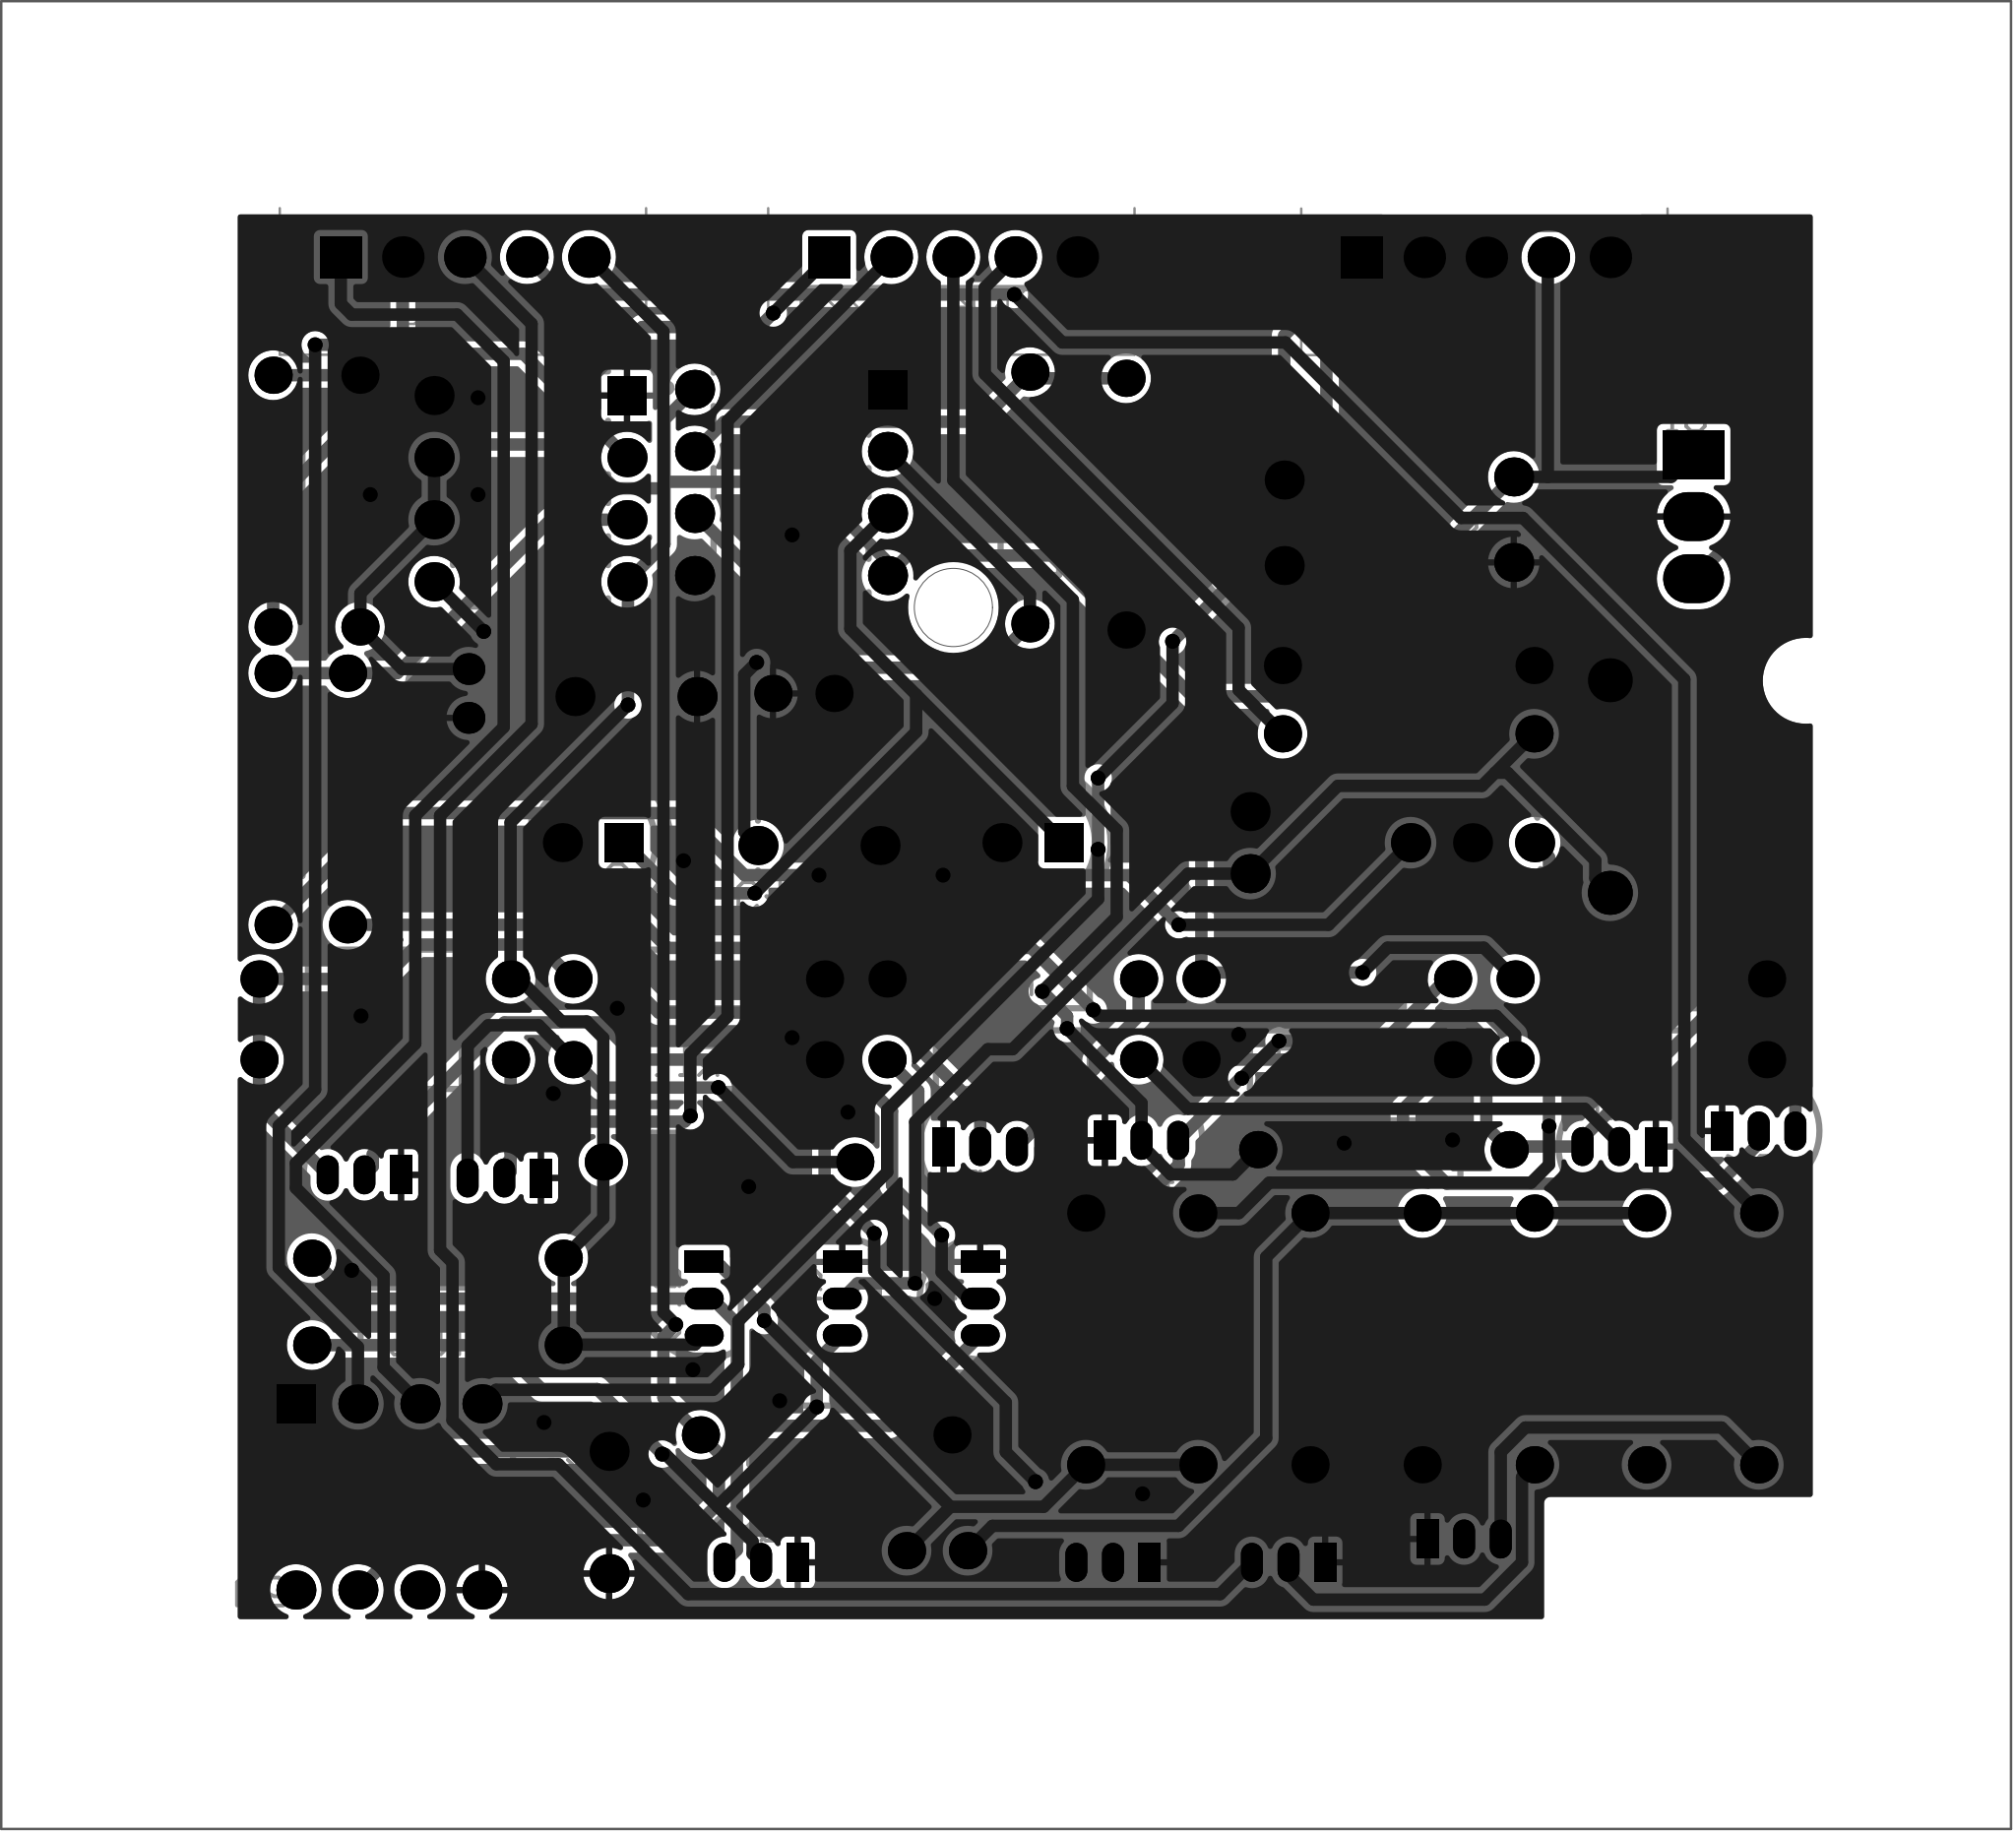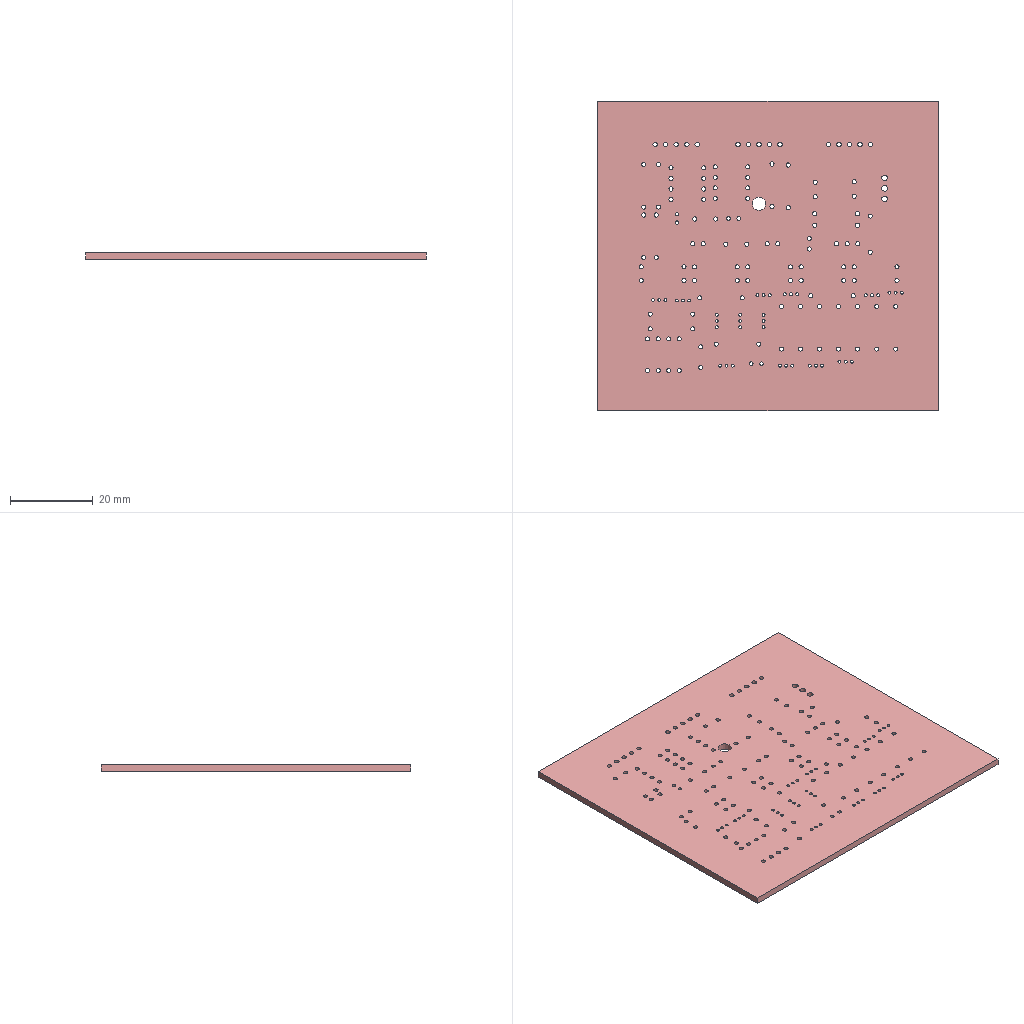Circuit board layout | Altium Designer | box 82.3 x 74.8 x 1.6 mm
Layer stack:
# Altium Designer layer stack of  (unit mm; dielectric type: 0 none, 1 core, 2 prepreg, 3 surface material)
index,name,kind,layer,copper_thickness_mm,dielectric_type,dielectric_thickness_mm,dielectric_material,dielectric_constant
0,Top Paste Mask Layer,other,,,,,,
1,Top Silkscreen Layer,other,,,,,,
2,Top Solder Mask Layer,dielectric,,,3,0.01,,3.3
3,Top Layer,copper,Top Layer,0.035,,,,
4,Dielectric1,dielectric,,,3,1.51,FR4,4.5
5,Bottom Layer,copper,Bottom Layer,0.035,,,,
6,Bottom Solder Mask Layer,dielectric,,,3,0.01,,3.3
7,Bottom Silkscreen Layer,other,,,,,,
8,Bottom Paste Mask Layer,other,,,,,,
# drill layer pairs: low layer,high layer
drill_pair,Top Layer,Bottom Layer
Part placement:
Designator,Comment,Layer,Footprint,Center-X(mm),Center-Y(mm),Rotation
C1,100uF,BottomLayer,CAP-TH_BD8.0-P3.50-D0.6-FD_1,131.784,123.433,270
C2,100uF,BottomLayer,CAP-TH_BD8.0-P3.50-D0.6-FD_1,122.386,123.306,270
C4,100nF,BottomLayer,CAP-TH_L5.0-W2.5-P5.00-D1.0,103.335,110.098,0
C9,100nF,BottomLayer,CAP-TH_L5.0-W2.5-P5.00-D1.0,94.742,82.804,270
C5,100UF,BottomLayer,CAP-TH_BD5.0-P2.00-D0.8-FD,88.985,116.321,270
R30,20kΩ,BottomLayer,Res_1/4W,103.632,85.979,180
C7,4.7uF,BottomLayer,CAP-TH_BD6.3-P2.50-D1.0-FD,120.989,110.217,90
C8,22uF,BottomLayer,CAP-TH_BD5.0-P2.5-D0.5-FD,108.17,81.239,0
D1,,BottomLayer,DO_1N4007,135.721,112.511,90
C6,100nF,BottomLayer,CAP-TH_L5.0-W2.5-P5.00-D1.0,95.843,116.194,0
U5,,BottomLayer,DIP-8_L9.9-W6.4-P2.54-LS7.6-BL,85.725,83.439,0
Q1,9013G,BottomLayer,TO-92-3_L4.9-W3.7-P1.27-L,84.721,96.62,180
Q2,9013G,BottomLayer,TO-92-3_L4.9-W3.7-P1.27-L,90.448,96.493,180
Q3,9013G,BottomLayer,TO-92-3_L4.9-W3.7-P1.27-L,109.94,97.779,0
Q4,9013G,BottomLayer,TO-92-3_L4.9-W3.7-P1.27-L,116.544,98.033,0
Q5,9013G,BottomLayer,TO-92-3_L4.9-W3.7-P1.27-L,136.102,97.779,180
Q6,9013G,BottomLayer,TO-92-3_L4.9-W3.7-P1.27-L,141.817,98.414,0
Q7,9013G,BottomLayer,TO-92-3_L4.9-W3.7-P1.27-L,104.288,91.556,270
Q8,9013G,BottomLayer,TO-92-3_L4.9-W3.7-P1.27-L,100.965,80.761,180
Q9,9013G,BottomLayer,TO-92-3_L4.9-W3.7-P1.27-L,109.94,91.556,270
Q10,9013G,BottomLayer,TO-92-3_L4.9-W3.7-P1.27-L,98.637,91.556,270
Q11,9013G,BottomLayer,TO-92-3_L4.9-W3.7-P1.27-L,115.374,80.761,180
Q12,9013G,BottomLayer,TO-92-3_L4.9-W3.7-P1.27-L,122.563,80.761,180
Q13,9013G,BottomLayer,TO-92-3_L4.9-W3.7-P1.27-L,129.752,81.717,0
R1,10kΩ,BottomLayer,Res_1/4W,115.909,124.068,270
R2,68kΩ,BottomLayer,Res_1/4W,111.972,124.322,90
R3,20kΩ,BottomLayer,Res_1/4W,80.984,124.195,90
R4,680kΩ,BottomLayer,Res_1/4W,84.54,124.195,90
R5,27kΩ,BottomLayer,Res_1/4W,84.032,112.003,90
R6,5.1kΩ,BottomLayer,Res_1/4W,80.984,112.003,90
R7,10kΩ,BottomLayer,Res_1/4W,85.556,104.637,0
R8,51kΩ,BottomLayer,Res_1/4W,85.556,101.335,180
R9,5.1kΩ,BottomLayer,Res_1/4W,99.653,97.144,180
R10,51kΩ,BottomLayer,Res_1/4W,98.414,104.637,180
R11,51kΩ,BottomLayer,Res_1/4W,98.414,101.335,180
R12,5.1kΩ,BottomLayer,Res_1/4W,111.273,104.637,180
R13,10kΩ,BottomLayer,Res_1/4W,124.132,104.637,180
R14,51kΩ,BottomLayer,Res_1/4W,111.273,101.335,180
R15,10kΩ,BottomLayer,Res_1/4W,136.991,104.637,180
R16,51kΩ,BottomLayer,Res_1/4W,87.715,89.651,180
R17,5.1kΩ,BottomLayer,Res_1/4W,87.715,93.207,180
R18,10kΩ,BottomLayer,Res_1/4W,136.991,101.335,180
R19,51kΩ,BottomLayer,Res_1/4W,124.132,101.335,180
R20,51kΩ,BottomLayer,Res_1/4W,126.45,97.652,0
R21,100Ω,BottomLayer,Res_1/4W,127.466,117.464,180
R22,5.1kΩ,BottomLayer,Res_1/4W,127.466,114.67,180
R23,20kΩ,BottomLayer,Res_1/4W,114.258,89.905,90
R24,27kΩ,BottomLayer,Res_1/4W,118.851,89.905,270
R25,20kΩ,BottomLayer,Res_1/4W,123.444,89.905,270
R26,2kΩ,BottomLayer,Res_1/4W,128.037,89.905,270
R27,2kΩ,BottomLayer,Res_1/4W,132.63,89.905,270
R28,27kΩ,BottomLayer,Res_1/4W,137.223,89.905,270
R29,300Ω,BottomLayer,Res_1/4W,141.817,89.905,270
U1,L7805,BottomLayer,TO-220AB-3_L10.4-W4.6-P2.54-L,139.15,123.56,270
U2,NE555,BottomLayer,PDIP-8_L9.6-W6.4-P2.54-LS7.9-BL-1,102.193,124.957,270
U4,NE555,BottomLayer,PDIP-8_L9.6-W6.4-P2.54-LS7.9-BL-1,91.525,124.703,270
H1,,BottomLayer,HDR-TH_5P-P2.54-V-M,88.835,134.183,0
H2,,BottomLayer,HDR-TH_5P-P2.54-V-M,108.835,134.183,0
H3,,BottomLayer,HDR-TH_5P-P2.54-V-M,130.663,134.169,0
D3,,BottomLayer,LED-TH_5mm,94.098,110.217,180
D2,,BottomLayer,LED-TH_5mm,112.098,110.217,180
OPTO1,38K infrared receiver, side-mounted,BottomLayer,OPTO-TH_3P-BD5.9-P2.54,130.098,110.213,270
C3,22uF,BottomLayer,CAP-TH_BD5.0-P2.5-D0.5-FD,102.701,116.321,180
Pad and via stacks:
# Altium Designer via and pad stacks of  (unit mm). Each distinct definition once, with the count of objects using it.
# via: kind,start_layer,end_layer,hole_mm,diameter_mm,mode(0 simple;1 top-mid-bottom;2 full stack),diameter_per_layer,count,example_net
# pad: kind,layer,hole_mm,hole_type(0 round;1 square;2 slot),plating,top_size,top_shape(1 round;2 rect;3 octagon;9 rounded rect),mid_size,bottom_size,mode,footprint,size_per_layer,count,example
pad,Multi-Layer,1,0,plated,1.6x1.6,1,1.6x1.6,1.6x1.6,0,CAP-TH_BD8.0-P3.50-D0.6-FD_1,,4,C1.2
pad,Multi-Layer,1,0,plated,1.6x1.6,1,1.6x1.6,1.6x1.6,0,CAP-TH_L5.0-W2.5-P5.00-D1.0,,6,C4.1
pad,Multi-Layer,0.8,0,plated,1.3x1.3,1,1.3x1.3,1.3x1.3,0,CAP-TH_BD5.0-P2.00-D0.8-FD,,2,C5.1
pad,Multi-Layer,1,0,plated,1.524x1.524,1,1.524x1.524,1.524x1.524,0,Res_1/4W,,60,R30.1
pad,Multi-Layer,1,0,plated,1.6x1.6,1,1.6x1.6,1.6x1.6,0,CAP-TH_BD6.3-P2.50-D1.0-FD,,2,C7.1
pad,Multi-Layer,0.9144,0,plated,1.524x1.524,1,1.524x1.524,1.524x1.524,0,CAP-TH_BD5.0-P2.5-D0.5-FD,,4,C8.1
pad,Multi-Layer,1,0,plated,1.8x1.8,1,1.8x1.8,1.8x1.8,0,DO_1N4007,,2,D1.1
pad,Multi-Layer,1,0,plated,1.6x1.6,1,1.6x1.6,1.6x1.6,0,DIP-8_L9.9-W6.4-P2.54-LS7.6-BL,,7,U5.8
pad,Multi-Layer,1,0,plated,1.6x1.6,2,1.6x1.6,1.6x1.6,0,DIP-8_L9.9-W6.4-P2.54-LS7.6-BL,,1,U5.1
pad,Multi-Layer,0.7,0,plated,0.9x1.6,1,0.9x1.6,0.9x1.6,0,TO-92-3_L4.9-W3.7-P1.27-L,,26,Q1.3
pad,Multi-Layer,0.7,0,plated,0.9x1.6,2,0.9x1.6,0.9x1.6,0,TO-92-3_L4.9-W3.7-P1.27-L,,13,Q1.1
pad,Multi-Layer,1.4,0,plated,2x2.5,1,2x2.5,2x2.5,0,TO-220AB-3_L10.4-W4.6-P2.54-L,,2,U1.2
pad,Multi-Layer,1.4,0,plated,2x2.5,2,2x2.5,2x2.5,0,TO-220AB-3_L10.4-W4.6-P2.54-L,,1,U1.1
pad,Multi-Layer,1,0,plated,1.6x1.6,1,1.6x1.6,1.6x1.6,0,PDIP-8_L9.6-W6.4-P2.54-LS7.9-BL-1,,14,U2.8
pad,Multi-Layer,1,0,plated,1.6x1.6,2,1.6x1.6,1.6x1.6,0,PDIP-8_L9.6-W6.4-P2.54-LS7.9-BL-1,,2,U2.1
pad,Multi-Layer,1.1,0,plated,1.7x1.7,2,1.7x1.7,1.7x1.7,0,HDR-TH_5P-P2.54-V-M,,3,H1.1
pad,Multi-Layer,1.1,0,plated,1.7x1.7,1,1.7x1.7,1.7x1.7,0,HDR-TH_5P-P2.54-V-M,,12,H1.2
pad,Multi-Layer,1,0,plated,1.6x1.6,2,1.6x1.6,1.6x1.6,0,LED-TH_5mm,,2,D3.1
pad,Multi-Layer,1,0,plated,1.6x1.6,1,1.6x1.6,1.6x1.6,0,LED-TH_5mm,,2,D3.2
pad,Multi-Layer,1,0,plated,1.6x1.6,1,1.6x1.6,1.6x1.6,0,OPTO-TH_3P-BD5.9-P2.54,,3,OPTO1.3
via,Top Layer,Bottom Layer,0.3048,0.6096,0,,29,$1N10142
via,Top Layer,Bottom Layer,0.3048,0.61,0,,22,OUTD
Copper pours:
name,layer,net,type(0 solid;1 hatched;2 none)
Bottom Layer-GND,Bottom Layer,GND,0
Top Layer-GND,Top Layer,GND,0
Design rules, without the lines most boards share:
# Altium Designer design rules of  (exported by Altium Designer, unit mm)
# columns: name | kind | enabled | priority | scope1 | scope2 | descriptor | typed fields (field=value)
copperThickness2oz | 0 | disabled | 1 | All | All | Clearance Constraint (Gap=6mil) (Disabled)(All),(All) | gap=0.1524
Plane_innerPlane | 0 | disabled | 2 | All | All | Clearance Constraint (Gap=6mil) (Disabled)(All),(All) | gap=0.1524
Copper_copperRegion | 0 | disabled | 3 | All | All | Clearance Constraint (Gap=6mil) (Disabled)(All),(All) | gap=0.1524
copperThickness1oz | 0 | enabled | 4 | All | All | Clearance Constraint (Gap=6mil) (All),(All) | gap=0.1524
otherClearance | 52 | enabled | 1 | All | All | Hole To Hole Clearance (Gap=11.8mil) (All),(All) | gap=0.2997
copperThickness1oz_2 | 2 | enabled | 2 | All | All | Width Constraint (Min=5mil) (Max=100mil) (Preferred=20mil) (All) |
viaSize | 11 | enabled | 1 | All | All | Routing Via (MinHoleWidth=11.8mil) (MaxHoleWidth=248mil) (PreferredHoleWidth=12mil) (MinWidth=19.7mil) (MaxWidth=393.7mil) (PreferedWidth=24mil) (All) | via_min_hole=0.2997 via_max_hole=6.299 via_preferred_diameter=0.6096 via_preferred_hole=0.3048